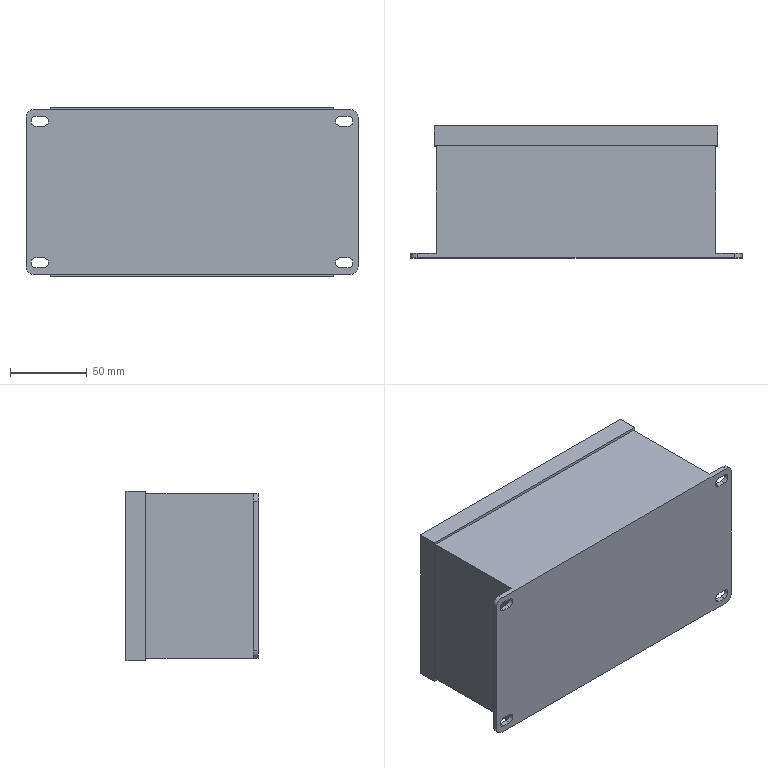Part | SolidWorks | features ICE 2, Extrusion 1 | 1 solid | 35 faces | box 216 x 86 x 110.411 mm | volume 1696161 mm3 | plane 23 | cylinder 12 | commonest cylinder face diameters 6.4 x8 10 x4
STEP:
#1=CARTESIAN_POINT('',(96.5,3.,42.8));
#2=VERTEX_POINT('',#1);
#3=CARTESIAN_POINT('',(96.5,3.,49.2));
#4=VERTEX_POINT('',#3);
#5=CARTESIAN_POINT('',(96.5,3.,46.));
#6=DIRECTION('',(0.,1.,0.));
#7=DIRECTION('',(0.,0.,1.));
#8=AXIS2_PLACEMENT_3D('',#5,#6,#7);
#9=CIRCLE('',#8,3.2);
#10=EDGE_CURVE('',#2,#4,#9,.T.);
#11=ORIENTED_EDGE('',*,*,#10,.F.);
#12=CARTESIAN_POINT('',(101.5,3.,42.8));
#13=VERTEX_POINT('',#12);
#14=CARTESIAN_POINT('',(96.5,3.,42.8));
#15=DIRECTION('',(-1.,0.,0.));
#16=VECTOR('',#15,1000.);
#17=LINE('',#14,#16);
#18=EDGE_CURVE('',#13,#2,#17,.T.);
#19=ORIENTED_EDGE('',*,*,#18,.F.);
#20=CARTESIAN_POINT('',(101.5,3.,49.2));
#21=VERTEX_POINT('',#20);
#22=CARTESIAN_POINT('',(101.5,3.,46.));
#23=DIRECTION('',(0.,1.,0.));
#24=DIRECTION('',(0.,0.,1.));
#25=AXIS2_PLACEMENT_3D('',#22,#23,#24);
#26=CIRCLE('',#25,3.2);
#27=EDGE_CURVE('',#21,#13,#26,.T.);
#28=ORIENTED_EDGE('',*,*,#27,.F.);
#29=CARTESIAN_POINT('',(96.5,3.,49.2));
#30=DIRECTION('',(1.,0.,0.));
#31=VECTOR('',#30,1000.);
#32=LINE('',#29,#31);
#33=EDGE_CURVE('',#4,#21,#32,.T.);
#34=ORIENTED_EDGE('',*,*,#33,.F.);
#35=EDGE_LOOP('',(#11,#19,#28,#34));
#36=FACE_BOUND('',#35,.T.);
#37=CARTESIAN_POINT('',(96.5,3.,-49.2));
#38=VERTEX_POINT('',#37);
#39=CARTESIAN_POINT('',(96.5,3.,-42.8));
#40=VERTEX_POINT('',#39);
#41=CARTESIAN_POINT('',(96.5,3.,-46.));
#42=DIRECTION('',(0.,1.,0.));
#43=DIRECTION('',(0.,0.,1.));
#44=AXIS2_PLACEMENT_3D('',#41,#42,#43);
#45=CIRCLE('',#44,3.2);
#46=EDGE_CURVE('',#38,#40,#45,.T.);
#47=ORIENTED_EDGE('',*,*,#46,.F.);
#48=CARTESIAN_POINT('',(101.5,3.,-49.2));
#49=VERTEX_POINT('',#48);
#50=CARTESIAN_POINT('',(96.5,3.,-49.2));
#51=DIRECTION('',(-1.,0.,0.));
#52=VECTOR('',#51,1000.);
#53=LINE('',#50,#52);
#54=EDGE_CURVE('',#49,#38,#53,.T.);
#55=ORIENTED_EDGE('',*,*,#54,.F.);
#56=CARTESIAN_POINT('',(101.5,3.,-42.8));
#57=VERTEX_POINT('',#56);
#58=CARTESIAN_POINT('',(101.5,3.,-46.));
#59=DIRECTION('',(0.,1.,0.));
#60=DIRECTION('',(0.,0.,1.));
#61=AXIS2_PLACEMENT_3D('',#58,#59,#60);
#62=CIRCLE('',#61,3.2);
#63=EDGE_CURVE('',#57,#49,#62,.T.);
#64=ORIENTED_EDGE('',*,*,#63,.F.);
#65=CARTESIAN_POINT('',(96.5,3.,-42.8));
#66=DIRECTION('',(1.,0.,0.));
#67=VECTOR('',#66,1000.);
#68=LINE('',#65,#67);
#69=EDGE_CURVE('',#40,#57,#68,.T.);
#70=ORIENTED_EDGE('',*,*,#69,.F.);
#71=EDGE_LOOP('',(#47,#55,#64,#70));
#72=FACE_BOUND('',#71,.T.);
#73=CARTESIAN_POINT('',(91.,3.,53.5));
#74=VERTEX_POINT('',#73);
#75=CARTESIAN_POINT('',(91.,3.,-53.5));
#76=VERTEX_POINT('',#75);
#77=CARTESIAN_POINT('',(91.,3.,53.5));
#78=DIRECTION('',(0.,0.,-1.));
#79=VECTOR('',#78,1000.);
#80=LINE('',#77,#79);
#81=EDGE_CURVE('',#74,#76,#80,.T.);
#82=ORIENTED_EDGE('',*,*,#81,.F.);
#83=CARTESIAN_POINT('',(103.,3.,53.5));
#84=VERTEX_POINT('',#83);
#85=CARTESIAN_POINT('',(-103.,3.,53.5));
#86=DIRECTION('',(1.,0.,0.));
#87=VECTOR('',#86,1000.);
#88=LINE('',#85,#87);
#89=EDGE_CURVE('',#74,#84,#88,.T.);
#90=ORIENTED_EDGE('',*,*,#89,.T.);
#91=CARTESIAN_POINT('',(108.,3.,48.5));
#92=VERTEX_POINT('',#91);
#93=CARTESIAN_POINT('',(103.,3.,48.5));
#94=DIRECTION('',(0.,1.,0.));
#95=DIRECTION('',(0.,0.,1.));
#96=AXIS2_PLACEMENT_3D('',#93,#94,#95);
#97=CIRCLE('',#96,5.);
#98=EDGE_CURVE('',#84,#92,#97,.T.);
#99=ORIENTED_EDGE('',*,*,#98,.T.);
#100=CARTESIAN_POINT('',(108.,3.,-48.5));
#101=VERTEX_POINT('',#100);
#102=CARTESIAN_POINT('',(108.,3.,48.5));
#103=DIRECTION('',(0.,0.,-1.));
#104=VECTOR('',#103,1000.);
#105=LINE('',#102,#104);
#106=EDGE_CURVE('',#92,#101,#105,.T.);
#107=ORIENTED_EDGE('',*,*,#106,.T.);
#108=CARTESIAN_POINT('',(103.,3.,-53.5));
#109=VERTEX_POINT('',#108);
#110=CARTESIAN_POINT('',(103.,3.,-48.5));
#111=DIRECTION('',(0.,1.,0.));
#112=DIRECTION('',(0.,0.,-1.));
#113=AXIS2_PLACEMENT_3D('',#110,#111,#112);
#114=CIRCLE('',#113,5.);
#115=EDGE_CURVE('',#101,#109,#114,.T.);
#116=ORIENTED_EDGE('',*,*,#115,.T.);
#117=CARTESIAN_POINT('',(-103.,3.,-53.5));
#118=DIRECTION('',(-1.,0.,0.));
#119=VECTOR('',#118,1000.);
#120=LINE('',#117,#119);
#121=EDGE_CURVE('',#109,#76,#120,.T.);
#122=ORIENTED_EDGE('',*,*,#121,.T.);
#123=EDGE_LOOP('',(#82,#90,#99,#107,#116,#122));
#124=FACE_OUTER_BOUND('',#123,.T.);
#125=CARTESIAN_POINT('',(-103.,3.,48.5));
#126=DIRECTION('',(0.,-1.,0.));
#127=DIRECTION('',(0.,0.,-1.));
#128=AXIS2_PLACEMENT_3D('',#125,#126,#127);
#129=PLANE('',#128);
#130=ADVANCED_FACE('',(#36,#72,#124),#129,.F.);
#131=CARTESIAN_POINT('',(-101.5,3.,-49.2));
#132=VERTEX_POINT('',#131);
#133=CARTESIAN_POINT('',(-101.5,3.,-42.8));
#134=VERTEX_POINT('',#133);
#135=CARTESIAN_POINT('',(-101.5,3.,-46.));
#136=DIRECTION('',(0.,1.,0.));
#137=DIRECTION('',(0.,0.,1.));
#138=AXIS2_PLACEMENT_3D('',#135,#136,#137);
#139=CIRCLE('',#138,3.2);
#140=EDGE_CURVE('',#132,#134,#139,.T.);
#141=ORIENTED_EDGE('',*,*,#140,.F.);
#142=CARTESIAN_POINT('',(-96.5,3.,-49.2));
#143=VERTEX_POINT('',#142);
#144=CARTESIAN_POINT('',(-101.5,3.,-49.2));
#145=DIRECTION('',(-1.,0.,0.));
#146=VECTOR('',#145,1000.);
#147=LINE('',#144,#146);
#148=EDGE_CURVE('',#143,#132,#147,.T.);
#149=ORIENTED_EDGE('',*,*,#148,.F.);
#150=CARTESIAN_POINT('',(-96.5,3.,-42.8));
#151=VERTEX_POINT('',#150);
#152=CARTESIAN_POINT('',(-96.5,3.,-46.));
#153=DIRECTION('',(0.,1.,0.));
#154=DIRECTION('',(0.,0.,1.));
#155=AXIS2_PLACEMENT_3D('',#152,#153,#154);
#156=CIRCLE('',#155,3.2);
#157=EDGE_CURVE('',#151,#143,#156,.T.);
#158=ORIENTED_EDGE('',*,*,#157,.F.);
#159=CARTESIAN_POINT('',(-101.5,3.,-42.8));
#160=DIRECTION('',(1.,0.,0.));
#161=VECTOR('',#160,1000.);
#162=LINE('',#159,#161);
#163=EDGE_CURVE('',#134,#151,#162,.T.);
#164=ORIENTED_EDGE('',*,*,#163,.F.);
#165=EDGE_LOOP('',(#141,#149,#158,#164));
#166=FACE_BOUND('',#165,.T.);
#167=CARTESIAN_POINT('',(-101.5,3.,42.8));
#168=VERTEX_POINT('',#167);
#169=CARTESIAN_POINT('',(-101.5,3.,49.2));
#170=VERTEX_POINT('',#169);
#171=CARTESIAN_POINT('',(-101.5,3.,46.));
#172=DIRECTION('',(0.,1.,0.));
#173=DIRECTION('',(0.,0.,1.));
#174=AXIS2_PLACEMENT_3D('',#171,#172,#173);
#175=CIRCLE('',#174,3.2);
#176=EDGE_CURVE('',#168,#170,#175,.T.);
#177=ORIENTED_EDGE('',*,*,#176,.F.);
#178=CARTESIAN_POINT('',(-96.5,3.,42.8));
#179=VERTEX_POINT('',#178);
#180=CARTESIAN_POINT('',(-101.5,3.,42.8));
#181=DIRECTION('',(-1.,0.,0.));
#182=VECTOR('',#181,1000.);
#183=LINE('',#180,#182);
#184=EDGE_CURVE('',#179,#168,#183,.T.);
#185=ORIENTED_EDGE('',*,*,#184,.F.);
#186=CARTESIAN_POINT('',(-96.5,3.,49.2));
#187=VERTEX_POINT('',#186);
#188=CARTESIAN_POINT('',(-96.5,3.,46.));
#189=DIRECTION('',(0.,1.,0.));
#190=DIRECTION('',(0.,0.,1.));
#191=AXIS2_PLACEMENT_3D('',#188,#189,#190);
#192=CIRCLE('',#191,3.2);
#193=EDGE_CURVE('',#187,#179,#192,.T.);
#194=ORIENTED_EDGE('',*,*,#193,.F.);
#195=CARTESIAN_POINT('',(-101.5,3.,49.2));
#196=DIRECTION('',(1.,0.,0.));
#197=VECTOR('',#196,1000.);
#198=LINE('',#195,#197);
#199=EDGE_CURVE('',#170,#187,#198,.T.);
#200=ORIENTED_EDGE('',*,*,#199,.F.);
#201=EDGE_LOOP('',(#177,#185,#194,#200));
#202=FACE_BOUND('',#201,.T.);
#203=CARTESIAN_POINT('',(-91.,3.,-53.5));
#204=VERTEX_POINT('',#203);
#205=CARTESIAN_POINT('',(-91.,3.,53.5));
#206=VERTEX_POINT('',#205);
#207=CARTESIAN_POINT('',(-91.,3.,53.5));
#208=DIRECTION('',(0.,0.,1.));
#209=VECTOR('',#208,1000.);
#210=LINE('',#207,#209);
#211=EDGE_CURVE('',#204,#206,#210,.T.);
#212=ORIENTED_EDGE('',*,*,#211,.F.);
#213=CARTESIAN_POINT('',(-103.,3.,-53.5));
#214=VERTEX_POINT('',#213);
#215=CARTESIAN_POINT('',(-103.,3.,-53.5));
#216=DIRECTION('',(-1.,0.,0.));
#217=VECTOR('',#216,1000.);
#218=LINE('',#215,#217);
#219=EDGE_CURVE('',#204,#214,#218,.T.);
#220=ORIENTED_EDGE('',*,*,#219,.T.);
#221=CARTESIAN_POINT('',(-108.,3.,-48.5));
#222=VERTEX_POINT('',#221);
#223=CARTESIAN_POINT('',(-103.,3.,-48.5));
#224=DIRECTION('',(0.,1.,0.));
#225=DIRECTION('',(0.,0.,-1.));
#226=AXIS2_PLACEMENT_3D('',#223,#224,#225);
#227=CIRCLE('',#226,5.);
#228=EDGE_CURVE('',#214,#222,#227,.T.);
#229=ORIENTED_EDGE('',*,*,#228,.T.);
#230=CARTESIAN_POINT('',(-108.,3.,48.5));
#231=VERTEX_POINT('',#230);
#232=CARTESIAN_POINT('',(-108.,3.,48.5));
#233=DIRECTION('',(0.,0.,1.));
#234=VECTOR('',#233,1000.);
#235=LINE('',#232,#234);
#236=EDGE_CURVE('',#222,#231,#235,.T.);
#237=ORIENTED_EDGE('',*,*,#236,.T.);
#238=CARTESIAN_POINT('',(-103.,3.,53.5));
#239=VERTEX_POINT('',#238);
#240=CARTESIAN_POINT('',(-103.,3.,48.5));
#241=DIRECTION('',(0.,1.,0.));
#242=DIRECTION('',(0.,0.,-1.));
#243=AXIS2_PLACEMENT_3D('',#240,#241,#242);
#244=CIRCLE('',#243,5.);
#245=EDGE_CURVE('',#231,#239,#244,.T.);
#246=ORIENTED_EDGE('',*,*,#245,.T.);
#247=CARTESIAN_POINT('',(-103.,3.,53.5));
#248=DIRECTION('',(1.,0.,0.));
#249=VECTOR('',#248,1000.);
#250=LINE('',#247,#249);
#251=EDGE_CURVE('',#239,#206,#250,.T.);
#252=ORIENTED_EDGE('',*,*,#251,.T.);
#253=EDGE_LOOP('',(#212,#220,#229,#237,#246,#252));
#254=FACE_OUTER_BOUND('',#253,.T.);
#255=CARTESIAN_POINT('',(-103.,3.,48.5));
#256=DIRECTION('',(0.,-1.,0.));
#257=DIRECTION('',(0.,0.,-1.));
#258=AXIS2_PLACEMENT_3D('',#255,#256,#257);
#259=PLANE('',#258);
#260=ADVANCED_FACE('',(#166,#202,#254),#259,.F.);
#261=CARTESIAN_POINT('',(-108.,0.,48.5));
#262=VERTEX_POINT('',#261);
#263=CARTESIAN_POINT('',(-103.,0.,53.5));
#264=VERTEX_POINT('',#263);
#265=CARTESIAN_POINT('',(-103.,0.,48.5));
#266=DIRECTION('',(0.,1.,0.));
#267=DIRECTION('',(0.,0.,-1.));
#268=AXIS2_PLACEMENT_3D('',#265,#266,#267);
#269=CIRCLE('',#268,5.);
#270=EDGE_CURVE('',#262,#264,#269,.T.);
#271=ORIENTED_EDGE('',*,*,#270,.F.);
#272=CARTESIAN_POINT('',(-108.,0.,-48.5));
#273=VERTEX_POINT('',#272);
#274=CARTESIAN_POINT('',(-108.,0.,48.5));
#275=DIRECTION('',(0.,0.,1.));
#276=VECTOR('',#275,1000.);
#277=LINE('',#274,#276);
#278=EDGE_CURVE('',#273,#262,#277,.T.);
#279=ORIENTED_EDGE('',*,*,#278,.F.);
#280=CARTESIAN_POINT('',(-103.,0.,-53.5));
#281=VERTEX_POINT('',#280);
#282=CARTESIAN_POINT('',(-103.,0.,-48.5));
#283=DIRECTION('',(0.,1.,0.));
#284=DIRECTION('',(0.,0.,-1.));
#285=AXIS2_PLACEMENT_3D('',#282,#283,#284);
#286=CIRCLE('',#285,5.);
#287=EDGE_CURVE('',#281,#273,#286,.T.);
#288=ORIENTED_EDGE('',*,*,#287,.F.);
#289=CARTESIAN_POINT('',(103.,0.,-53.5));
#290=VERTEX_POINT('',#289);
#291=CARTESIAN_POINT('',(-103.,0.,-53.5));
#292=DIRECTION('',(-1.,0.,0.));
#293=VECTOR('',#292,1000.);
#294=LINE('',#291,#293);
#295=EDGE_CURVE('',#290,#281,#294,.T.);
#296=ORIENTED_EDGE('',*,*,#295,.F.);
#297=CARTESIAN_POINT('',(108.,0.,-48.5));
#298=VERTEX_POINT('',#297);
#299=CARTESIAN_POINT('',(103.,0.,-48.5));
#300=DIRECTION('',(0.,1.,0.));
#301=DIRECTION('',(0.,0.,-1.));
#302=AXIS2_PLACEMENT_3D('',#299,#300,#301);
#303=CIRCLE('',#302,5.);
#304=EDGE_CURVE('',#298,#290,#303,.T.);
#305=ORIENTED_EDGE('',*,*,#304,.F.);
#306=CARTESIAN_POINT('',(108.,0.,48.5));
#307=VERTEX_POINT('',#306);
#308=CARTESIAN_POINT('',(108.,0.,48.5));
#309=DIRECTION('',(0.,0.,-1.));
#310=VECTOR('',#309,1000.);
#311=LINE('',#308,#310);
#312=EDGE_CURVE('',#307,#298,#311,.T.);
#313=ORIENTED_EDGE('',*,*,#312,.F.);
#314=CARTESIAN_POINT('',(103.,0.,53.5));
#315=VERTEX_POINT('',#314);
#316=CARTESIAN_POINT('',(103.,0.,48.5));
#317=DIRECTION('',(0.,1.,0.));
#318=DIRECTION('',(0.,0.,1.));
#319=AXIS2_PLACEMENT_3D('',#316,#317,#318);
#320=CIRCLE('',#319,5.);
#321=EDGE_CURVE('',#315,#307,#320,.T.);
#322=ORIENTED_EDGE('',*,*,#321,.F.);
#323=CARTESIAN_POINT('',(-103.,0.,53.5));
#324=DIRECTION('',(1.,0.,0.));
#325=VECTOR('',#324,1000.);
#326=LINE('',#323,#325);
#327=EDGE_CURVE('',#264,#315,#326,.T.);
#328=ORIENTED_EDGE('',*,*,#327,.F.);
#329=EDGE_LOOP('',(#271,#279,#288,#296,#305,#313,#322,#328));
#330=FACE_OUTER_BOUND('',#329,.T.);
#331=CARTESIAN_POINT('',(-96.5,0.,-49.2));
#332=VERTEX_POINT('',#331);
#333=CARTESIAN_POINT('',(-101.5,0.,-49.2));
#334=VERTEX_POINT('',#333);
#335=CARTESIAN_POINT('',(-101.5,0.,-49.2));
#336=DIRECTION('',(-1.,0.,0.));
#337=VECTOR('',#336,1000.);
#338=LINE('',#335,#337);
#339=EDGE_CURVE('',#332,#334,#338,.T.);
#340=ORIENTED_EDGE('',*,*,#339,.T.);
#341=CARTESIAN_POINT('',(-101.5,0.,-42.8));
#342=VERTEX_POINT('',#341);
#343=CARTESIAN_POINT('',(-101.5,0.,-46.));
#344=DIRECTION('',(0.,1.,0.));
#345=DIRECTION('',(0.,0.,1.));
#346=AXIS2_PLACEMENT_3D('',#343,#344,#345);
#347=CIRCLE('',#346,3.2);
#348=EDGE_CURVE('',#334,#342,#347,.T.);
#349=ORIENTED_EDGE('',*,*,#348,.T.);
#350=CARTESIAN_POINT('',(-96.5,0.,-42.8));
#351=VERTEX_POINT('',#350);
#352=CARTESIAN_POINT('',(-101.5,0.,-42.8));
#353=DIRECTION('',(1.,0.,0.));
#354=VECTOR('',#353,1000.);
#355=LINE('',#352,#354);
#356=EDGE_CURVE('',#342,#351,#355,.T.);
#357=ORIENTED_EDGE('',*,*,#356,.T.);
#358=CARTESIAN_POINT('',(-96.5,0.,-46.));
#359=DIRECTION('',(0.,1.,0.));
#360=DIRECTION('',(0.,0.,1.));
#361=AXIS2_PLACEMENT_3D('',#358,#359,#360);
#362=CIRCLE('',#361,3.2);
#363=EDGE_CURVE('',#351,#332,#362,.T.);
#364=ORIENTED_EDGE('',*,*,#363,.T.);
#365=EDGE_LOOP('',(#340,#349,#357,#364));
#366=FACE_BOUND('',#365,.T.);
#367=CARTESIAN_POINT('',(101.5,0.,-49.2));
#368=VERTEX_POINT('',#367);
#369=CARTESIAN_POINT('',(96.5,0.,-49.2));
#370=VERTEX_POINT('',#369);
#371=CARTESIAN_POINT('',(96.5,0.,-49.2));
#372=DIRECTION('',(-1.,0.,0.));
#373=VECTOR('',#372,1000.);
#374=LINE('',#371,#373);
#375=EDGE_CURVE('',#368,#370,#374,.T.);
#376=ORIENTED_EDGE('',*,*,#375,.T.);
#377=CARTESIAN_POINT('',(96.5,0.,-42.8));
#378=VERTEX_POINT('',#377);
#379=CARTESIAN_POINT('',(96.5,0.,-46.));
#380=DIRECTION('',(0.,1.,0.));
#381=DIRECTION('',(0.,0.,1.));
#382=AXIS2_PLACEMENT_3D('',#379,#380,#381);
#383=CIRCLE('',#382,3.2);
#384=EDGE_CURVE('',#370,#378,#383,.T.);
#385=ORIENTED_EDGE('',*,*,#384,.T.);
#386=CARTESIAN_POINT('',(101.5,0.,-42.8));
#387=VERTEX_POINT('',#386);
#388=CARTESIAN_POINT('',(96.5,0.,-42.8));
#389=DIRECTION('',(1.,0.,0.));
#390=VECTOR('',#389,1000.);
#391=LINE('',#388,#390);
#392=EDGE_CURVE('',#378,#387,#391,.T.);
#393=ORIENTED_EDGE('',*,*,#392,.T.);
#394=CARTESIAN_POINT('',(101.5,0.,-46.));
#395=DIRECTION('',(0.,1.,0.));
#396=DIRECTION('',(0.,0.,1.));
#397=AXIS2_PLACEMENT_3D('',#394,#395,#396);
#398=CIRCLE('',#397,3.2);
#399=EDGE_CURVE('',#387,#368,#398,.T.);
#400=ORIENTED_EDGE('',*,*,#399,.T.);
#401=EDGE_LOOP('',(#376,#385,#393,#400));
#402=FACE_BOUND('',#401,.T.);
#403=CARTESIAN_POINT('',(-96.5,0.,42.8));
#404=VERTEX_POINT('',#403);
#405=CARTESIAN_POINT('',(-101.5,0.,42.8));
#406=VERTEX_POINT('',#405);
#407=CARTESIAN_POINT('',(-101.5,0.,42.8));
#408=DIRECTION('',(-1.,0.,0.));
#409=VECTOR('',#408,1000.);
#410=LINE('',#407,#409);
#411=EDGE_CURVE('',#404,#406,#410,.T.);
#412=ORIENTED_EDGE('',*,*,#411,.T.);
#413=CARTESIAN_POINT('',(-101.5,0.,49.2));
#414=VERTEX_POINT('',#413);
#415=CARTESIAN_POINT('',(-101.5,0.,46.));
#416=DIRECTION('',(0.,1.,0.));
#417=DIRECTION('',(0.,0.,1.));
#418=AXIS2_PLACEMENT_3D('',#415,#416,#417);
#419=CIRCLE('',#418,3.2);
#420=EDGE_CURVE('',#406,#414,#419,.T.);
#421=ORIENTED_EDGE('',*,*,#420,.T.);
#422=CARTESIAN_POINT('',(-96.5,0.,49.2));
#423=VERTEX_POINT('',#422);
#424=CARTESIAN_POINT('',(-101.5,0.,49.2));
#425=DIRECTION('',(1.,0.,0.));
#426=VECTOR('',#425,1000.);
#427=LINE('',#424,#426);
#428=EDGE_CURVE('',#414,#423,#427,.T.);
#429=ORIENTED_EDGE('',*,*,#428,.T.);
#430=CARTESIAN_POINT('',(-96.5,0.,46.));
#431=DIRECTION('',(0.,1.,0.));
#432=DIRECTION('',(0.,0.,1.));
#433=AXIS2_PLACEMENT_3D('',#430,#431,#432);
#434=CIRCLE('',#433,3.2);
#435=EDGE_CURVE('',#423,#404,#434,.T.);
#436=ORIENTED_EDGE('',*,*,#435,.T.);
#437=EDGE_LOOP('',(#412,#421,#429,#436));
#438=FACE_BOUND('',#437,.T.);
#439=CARTESIAN_POINT('',(101.5,0.,42.8));
#440=VERTEX_POINT('',#439);
#441=CARTESIAN_POINT('',(96.5,0.,42.8));
#442=VERTEX_POINT('',#441);
#443=CARTESIAN_POINT('',(96.5,0.,42.8));
#444=DIRECTION('',(-1.,0.,0.));
#445=VECTOR('',#444,1000.);
#446=LINE('',#443,#445);
#447=EDGE_CURVE('',#440,#442,#446,.T.);
#448=ORIENTED_EDGE('',*,*,#447,.T.);
#449=CARTESIAN_POINT('',(96.5,0.,49.2));
#450=VERTEX_POINT('',#449);
#451=CARTESIAN_POINT('',(96.5,0.,46.));
#452=DIRECTION('',(0.,1.,0.));
#453=DIRECTION('',(0.,0.,1.));
#454=AXIS2_PLACEMENT_3D('',#451,#452,#453);
#455=CIRCLE('',#454,3.2);
#456=EDGE_CURVE('',#442,#450,#455,.T.);
#457=ORIENTED_EDGE('',*,*,#456,.T.);
#458=CARTESIAN_POINT('',(101.5,0.,49.2));
#459=VERTEX_POINT('',#458);
#460=CARTESIAN_POINT('',(96.5,0.,49.2));
#461=DIRECTION('',(1.,0.,0.));
#462=VECTOR('',#461,1000.);
#463=LINE('',#460,#462);
#464=EDGE_CURVE('',#450,#459,#463,.T.);
#465=ORIENTED_EDGE('',*,*,#464,.T.);
#466=CARTESIAN_POINT('',(101.5,0.,46.));
#467=DIRECTION('',(0.,1.,0.));
#468=DIRECTION('',(0.,0.,1.));
#469=AXIS2_PLACEMENT_3D('',#466,#467,#468);
#470=CIRCLE('',#469,3.2);
#471=EDGE_CURVE('',#459,#440,#470,.T.);
#472=ORIENTED_EDGE('',*,*,#471,.T.);
#473=EDGE_LOOP('',(#448,#457,#465,#472));
#474=FACE_BOUND('',#473,.T.);
#475=CARTESIAN_POINT('',(-103.,0.,48.5));
#476=DIRECTION('',(0.,-1.,0.));
#477=DIRECTION('',(0.,0.,-1.));
#478=AXIS2_PLACEMENT_3D('',#475,#476,#477);
#479=PLANE('',#478);
#480=ADVANCED_FACE('',(#330,#366,#402,#438,#474),#479,.T.);
#481=ORIENTED_EDGE('',*,*,#270,.T.);
#482=CARTESIAN_POINT('',(-103.,3.,53.5));
#483=DIRECTION('',(0.,-1.,0.));
#484=VECTOR('',#483,1000.);
#485=LINE('',#482,#484);
#486=EDGE_CURVE('',#239,#264,#485,.T.);
#487=ORIENTED_EDGE('',*,*,#486,.F.);
#488=ORIENTED_EDGE('',*,*,#245,.F.);
#489=CARTESIAN_POINT('',(-108.,3.,48.5));
#490=DIRECTION('',(0.,-1.,0.));
#491=VECTOR('',#490,1000.);
#492=LINE('',#489,#491);
#493=EDGE_CURVE('',#231,#262,#492,.T.);
#494=ORIENTED_EDGE('',*,*,#493,.T.);
#495=EDGE_LOOP('',(#481,#487,#488,#494));
#496=FACE_OUTER_BOUND('',#495,.T.);
#497=CARTESIAN_POINT('',(-103.,3.,48.5));
#498=DIRECTION('',(0.,-1.,0.));
#499=DIRECTION('',(0.,0.,-1.));
#500=AXIS2_PLACEMENT_3D('',#497,#498,#499);
#501=CYLINDRICAL_SURFACE('',#500,5.);
#502=ADVANCED_FACE('',(#496),#501,.T.);
#503=ORIENTED_EDGE('',*,*,#327,.T.);
#504=CARTESIAN_POINT('',(103.,3.,53.5));
#505=DIRECTION('',(0.,-1.,0.));
#506=VECTOR('',#505,1000.);
#507=LINE('',#504,#506);
#508=EDGE_CURVE('',#84,#315,#507,.T.);
#509=ORIENTED_EDGE('',*,*,#508,.F.);
#510=ORIENTED_EDGE('',*,*,#89,.F.);
#511=CARTESIAN_POINT('',(91.,73.,53.5));
#512=VERTEX_POINT('',#511);
#513=CARTESIAN_POINT('',(91.,73.,53.5));
#514=DIRECTION('',(0.,-1.,0.));
#515=VECTOR('',#514,1000.);
#516=LINE('',#513,#515);
#517=EDGE_CURVE('',#512,#74,#516,.T.);
#518=ORIENTED_EDGE('',*,*,#517,.F.);
#519=CARTESIAN_POINT('',(-91.,73.,53.5));
#520=VERTEX_POINT('',#519);
#521=CARTESIAN_POINT('',(-91.,73.,53.5));
#522=DIRECTION('',(1.,0.,0.));
#523=VECTOR('',#522,1000.);
#524=LINE('',#521,#523);
#525=EDGE_CURVE('',#520,#512,#524,.T.);
#526=ORIENTED_EDGE('',*,*,#525,.F.);
#527=CARTESIAN_POINT('',(-91.,73.,53.5));
#528=DIRECTION('',(0.,-1.,0.));
#529=VECTOR('',#528,1000.);
#530=LINE('',#527,#529);
#531=EDGE_CURVE('',#520,#206,#530,.T.);
#532=ORIENTED_EDGE('',*,*,#531,.T.);
#533=ORIENTED_EDGE('',*,*,#251,.F.);
#534=ORIENTED_EDGE('',*,*,#486,.T.);
#535=EDGE_LOOP('',(#503,#509,#510,#518,#526,#532,#533,#534));
#536=FACE_OUTER_BOUND('',#535,.T.);
#537=CARTESIAN_POINT('',(-103.,3.,53.5));
#538=DIRECTION('',(0.,0.,-1.));
#539=DIRECTION('',(-1.,0.,0.));
#540=AXIS2_PLACEMENT_3D('',#537,#538,#539);
#541=PLANE('',#540);
#542=ADVANCED_FACE('',(#536),#541,.F.);
#543=ORIENTED_EDGE('',*,*,#321,.T.);
#544=CARTESIAN_POINT('',(108.,3.,48.5));
#545=DIRECTION('',(0.,-1.,0.));
#546=VECTOR('',#545,1000.);
#547=LINE('',#544,#546);
#548=EDGE_CURVE('',#92,#307,#547,.T.);
#549=ORIENTED_EDGE('',*,*,#548,.F.);
#550=ORIENTED_EDGE('',*,*,#98,.F.);
#551=ORIENTED_EDGE('',*,*,#508,.T.);
#552=EDGE_LOOP('',(#543,#549,#550,#551));
#553=FACE_OUTER_BOUND('',#552,.T.);
#554=CARTESIAN_POINT('',(103.,3.,48.5));
#555=DIRECTION('',(0.,-1.,0.));
#556=DIRECTION('',(0.,0.,-1.));
#557=AXIS2_PLACEMENT_3D('',#554,#555,#556);
#558=CYLINDRICAL_SURFACE('',#557,5.);
#559=ADVANCED_FACE('',(#553),#558,.T.);
#560=ORIENTED_EDGE('',*,*,#312,.T.);
#561=CARTESIAN_POINT('',(108.,3.,-48.5));
#562=DIRECTION('',(0.,-1.,0.));
#563=VECTOR('',#562,1000.);
#564=LINE('',#561,#563);
#565=EDGE_CURVE('',#101,#298,#564,.T.);
#566=ORIENTED_EDGE('',*,*,#565,.F.);
#567=ORIENTED_EDGE('',*,*,#106,.F.);
#568=ORIENTED_EDGE('',*,*,#548,.T.);
#569=EDGE_LOOP('',(#560,#566,#567,#568));
#570=FACE_OUTER_BOUND('',#569,.T.);
#571=CARTESIAN_POINT('',(108.,3.,48.5));
#572=DIRECTION('',(-1.,0.,0.));
#573=DIRECTION('',(0.,0.,1.));
#574=AXIS2_PLACEMENT_3D('',#571,#572,#573);
#575=PLANE('',#574);
#576=ADVANCED_FACE('',(#570),#575,.F.);
#577=ORIENTED_EDGE('',*,*,#304,.T.);
#578=CARTESIAN_POINT('',(103.,3.,-53.5));
#579=DIRECTION('',(0.,-1.,0.));
#580=VECTOR('',#579,1000.);
#581=LINE('',#578,#580);
#582=EDGE_CURVE('',#109,#290,#581,.T.);
#583=ORIENTED_EDGE('',*,*,#582,.F.);
#584=ORIENTED_EDGE('',*,*,#115,.F.);
#585=ORIENTED_EDGE('',*,*,#565,.T.);
#586=EDGE_LOOP('',(#577,#583,#584,#585));
#587=FACE_OUTER_BOUND('',#586,.T.);
#588=CARTESIAN_POINT('',(103.,3.,-48.5));
#589=DIRECTION('',(0.,-1.,0.));
#590=DIRECTION('',(0.,0.,-1.));
#591=AXIS2_PLACEMENT_3D('',#588,#589,#590);
#592=CYLINDRICAL_SURFACE('',#591,5.);
#593=ADVANCED_FACE('',(#587),#592,.T.);
#594=ORIENTED_EDGE('',*,*,#295,.T.);
#595=CARTESIAN_POINT('',(-103.,3.,-53.5));
#596=DIRECTION('',(0.,-1.,0.));
#597=VECTOR('',#596,1000.);
#598=LINE('',#595,#597);
#599=EDGE_CURVE('',#214,#281,#598,.T.);
#600=ORIENTED_EDGE('',*,*,#599,.F.);
#601=ORIENTED_EDGE('',*,*,#219,.F.);
#602=CARTESIAN_POINT('',(-91.,73.,-53.5));
#603=VERTEX_POINT('',#602);
#604=CARTESIAN_POINT('',(-91.,73.,-53.5));
#605=DIRECTION('',(0.,-1.,0.));
#606=VECTOR('',#605,1000.);
#607=LINE('',#604,#606);
#608=EDGE_CURVE('',#603,#204,#607,.T.);
#609=ORIENTED_EDGE('',*,*,#608,.F.);
#610=CARTESIAN_POINT('',(91.,73.,-53.5));
#611=VERTEX_POINT('',#610);
#612=CARTESIAN_POINT('',(-91.,73.,-53.5));
#613=DIRECTION('',(-1.,0.,0.));
#614=VECTOR('',#613,1000.);
#615=LINE('',#612,#614);
#616=EDGE_CURVE('',#611,#603,#615,.T.);
#617=ORIENTED_EDGE('',*,*,#616,.F.);
#618=CARTESIAN_POINT('',(91.,73.,-53.5));
#619=DIRECTION('',(0.,-1.,0.));
#620=VECTOR('',#619,1000.);
#621=LINE('',#618,#620);
#622=EDGE_CURVE('',#611,#76,#621,.T.);
#623=ORIENTED_EDGE('',*,*,#622,.T.);
#624=ORIENTED_EDGE('',*,*,#121,.F.);
#625=ORIENTED_EDGE('',*,*,#582,.T.);
#626=EDGE_LOOP('',(#594,#600,#601,#609,#617,#623,#624,#625));
#627=FACE_OUTER_BOUND('',#626,.T.);
#628=CARTESIAN_POINT('',(-103.,3.,-53.5));
#629=DIRECTION('',(0.,0.,1.));
#630=DIRECTION('',(1.,0.,0.));
#631=AXIS2_PLACEMENT_3D('',#628,#629,#630);
#632=PLANE('',#631);
#633=ADVANCED_FACE('',(#627),#632,.F.);
#634=ORIENTED_EDGE('',*,*,#287,.T.);
#635=CARTESIAN_POINT('',(-108.,3.,-48.5));
#636=DIRECTION('',(0.,-1.,0.));
#637=VECTOR('',#636,1000.);
#638=LINE('',#635,#637);
#639=EDGE_CURVE('',#222,#273,#638,.T.);
#640=ORIENTED_EDGE('',*,*,#639,.F.);
#641=ORIENTED_EDGE('',*,*,#228,.F.);
#642=ORIENTED_EDGE('',*,*,#599,.T.);
#643=EDGE_LOOP('',(#634,#640,#641,#642));
#644=FACE_OUTER_BOUND('',#643,.T.);
#645=CARTESIAN_POINT('',(-103.,3.,-48.5));
#646=DIRECTION('',(0.,-1.,0.));
#647=DIRECTION('',(0.,0.,-1.));
#648=AXIS2_PLACEMENT_3D('',#645,#646,#647);
#649=CYLINDRICAL_SURFACE('',#648,5.);
#650=ADVANCED_FACE('',(#644),#649,.T.);
#651=ORIENTED_EDGE('',*,*,#278,.T.);
#652=ORIENTED_EDGE('',*,*,#493,.F.);
#653=ORIENTED_EDGE('',*,*,#236,.F.);
#654=ORIENTED_EDGE('',*,*,#639,.T.);
#655=EDGE_LOOP('',(#651,#652,#653,#654));
#656=FACE_OUTER_BOUND('',#655,.T.);
#657=CARTESIAN_POINT('',(-108.,3.,48.5));
#658=DIRECTION('',(1.,0.,0.));
#659=DIRECTION('',(0.,0.,-1.));
#660=AXIS2_PLACEMENT_3D('',#657,#658,#659);
#661=PLANE('',#660);
#662=ADVANCED_FACE('',(#656),#661,.F.);
#663=ORIENTED_EDGE('',*,*,#348,.F.);
#664=CARTESIAN_POINT('',(-101.5,3.,-49.2));
#665=DIRECTION('',(0.,-1.,0.));
#666=VECTOR('',#665,1000.);
#667=LINE('',#664,#666);
#668=EDGE_CURVE('',#132,#334,#667,.T.);
#669=ORIENTED_EDGE('',*,*,#668,.F.);
#670=ORIENTED_EDGE('',*,*,#140,.T.);
#671=CARTESIAN_POINT('',(-101.5,3.,-42.8));
#672=DIRECTION('',(0.,-1.,0.));
#673=VECTOR('',#672,1000.);
#674=LINE('',#671,#673);
#675=EDGE_CURVE('',#134,#342,#674,.T.);
#676=ORIENTED_EDGE('',*,*,#675,.T.);
#677=EDGE_LOOP('',(#663,#669,#670,#676));
#678=FACE_OUTER_BOUND('',#677,.T.);
#679=CARTESIAN_POINT('',(-101.5,3.,-46.));
#680=DIRECTION('',(0.,-1.,0.));
#681=DIRECTION('',(0.,0.,-1.));
#682=AXIS2_PLACEMENT_3D('',#679,#680,#681);
#683=CYLINDRICAL_SURFACE('',#682,3.2);
#684=ADVANCED_FACE('',(#678),#683,.F.);
#685=ORIENTED_EDGE('',*,*,#356,.F.);
#686=ORIENTED_EDGE('',*,*,#675,.F.);
#687=ORIENTED_EDGE('',*,*,#163,.T.);
#688=CARTESIAN_POINT('',(-96.5,3.,-42.8));
#689=DIRECTION('',(0.,-1.,0.));
#690=VECTOR('',#689,1000.);
#691=LINE('',#688,#690);
#692=EDGE_CURVE('',#151,#351,#691,.T.);
#693=ORIENTED_EDGE('',*,*,#692,.T.);
#694=EDGE_LOOP('',(#685,#686,#687,#693));
#695=FACE_OUTER_BOUND('',#694,.T.);
#696=CARTESIAN_POINT('',(-101.5,3.,-42.8));
#697=DIRECTION('',(0.,0.,-1.));
#698=DIRECTION('',(-1.,0.,0.));
#699=AXIS2_PLACEMENT_3D('',#696,#697,#698);
#700=PLANE('',#699);
#701=ADVANCED_FACE('',(#695),#700,.T.);
#702=ORIENTED_EDGE('',*,*,#363,.F.);
#703=ORIENTED_EDGE('',*,*,#692,.F.);
#704=ORIENTED_EDGE('',*,*,#157,.T.);
#705=CARTESIAN_POINT('',(-96.5,3.,-49.2));
#706=DIRECTION('',(0.,-1.,0.));
#707=VECTOR('',#706,1000.);
#708=LINE('',#705,#707);
#709=EDGE_CURVE('',#143,#332,#708,.T.);
#710=ORIENTED_EDGE('',*,*,#709,.T.);
#711=EDGE_LOOP('',(#702,#703,#704,#710));
#712=FACE_OUTER_BOUND('',#711,.T.);
#713=CARTESIAN_POINT('',(-96.5,3.,-46.));
#714=DIRECTION('',(0.,-1.,0.));
#715=DIRECTION('',(0.,0.,-1.));
#716=AXIS2_PLACEMENT_3D('',#713,#714,#715);
#717=CYLINDRICAL_SURFACE('',#716,3.2);
#718=ADVANCED_FACE('',(#712),#717,.F.);
#719=ORIENTED_EDGE('',*,*,#339,.F.);
#720=ORIENTED_EDGE('',*,*,#709,.F.);
#721=ORIENTED_EDGE('',*,*,#148,.T.);
#722=ORIENTED_EDGE('',*,*,#668,.T.);
#723=EDGE_LOOP('',(#719,#720,#721,#722));
#724=FACE_OUTER_BOUND('',#723,.T.);
#725=CARTESIAN_POINT('',(-101.5,3.,-49.2));
#726=DIRECTION('',(0.,0.,1.));
#727=DIRECTION('',(1.,0.,0.));
#728=AXIS2_PLACEMENT_3D('',#725,#726,#727);
#729=PLANE('',#728);
#730=ADVANCED_FACE('',(#724),#729,.T.);
#731=ORIENTED_EDGE('',*,*,#384,.F.);
#732=CARTESIAN_POINT('',(96.5,3.,-49.2));
#733=DIRECTION('',(0.,-1.,0.));
#734=VECTOR('',#733,1000.);
#735=LINE('',#732,#734);
#736=EDGE_CURVE('',#38,#370,#735,.T.);
#737=ORIENTED_EDGE('',*,*,#736,.F.);
#738=ORIENTED_EDGE('',*,*,#46,.T.);
#739=CARTESIAN_POINT('',(96.5,3.,-42.8));
#740=DIRECTION('',(0.,-1.,0.));
#741=VECTOR('',#740,1000.);
#742=LINE('',#739,#741);
#743=EDGE_CURVE('',#40,#378,#742,.T.);
#744=ORIENTED_EDGE('',*,*,#743,.T.);
#745=EDGE_LOOP('',(#731,#737,#738,#744));
#746=FACE_OUTER_BOUND('',#745,.T.);
#747=CARTESIAN_POINT('',(96.5,3.,-46.));
#748=DIRECTION('',(0.,-1.,0.));
#749=DIRECTION('',(0.,0.,-1.));
#750=AXIS2_PLACEMENT_3D('',#747,#748,#749);
#751=CYLINDRICAL_SURFACE('',#750,3.2);
#752=ADVANCED_FACE('',(#746),#751,.F.);
#753=ORIENTED_EDGE('',*,*,#392,.F.);
#754=ORIENTED_EDGE('',*,*,#743,.F.);
#755=ORIENTED_EDGE('',*,*,#69,.T.);
#756=CARTESIAN_POINT('',(101.5,3.,-42.8));
#757=DIRECTION('',(0.,-1.,0.));
#758=VECTOR('',#757,1000.);
#759=LINE('',#756,#758);
#760=EDGE_CURVE('',#57,#387,#759,.T.);
#761=ORIENTED_EDGE('',*,*,#760,.T.);
#762=EDGE_LOOP('',(#753,#754,#755,#761));
#763=FACE_OUTER_BOUND('',#762,.T.);
#764=CARTESIAN_POINT('',(96.5,3.,-42.8));
#765=DIRECTION('',(0.,0.,-1.));
#766=DIRECTION('',(-1.,0.,0.));
#767=AXIS2_PLACEMENT_3D('',#764,#765,#766);
#768=PLANE('',#767);
#769=ADVANCED_FACE('',(#763),#768,.T.);
#770=ORIENTED_EDGE('',*,*,#399,.F.);
#771=ORIENTED_EDGE('',*,*,#760,.F.);
#772=ORIENTED_EDGE('',*,*,#63,.T.);
#773=CARTESIAN_POINT('',(101.5,3.,-49.2));
#774=DIRECTION('',(0.,-1.,0.));
#775=VECTOR('',#774,1000.);
#776=LINE('',#773,#775);
#777=EDGE_CURVE('',#49,#368,#776,.T.);
#778=ORIENTED_EDGE('',*,*,#777,.T.);
#779=EDGE_LOOP('',(#770,#771,#772,#778));
#780=FACE_OUTER_BOUND('',#779,.T.);
#781=CARTESIAN_POINT('',(101.5,3.,-46.));
#782=DIRECTION('',(0.,-1.,0.));
#783=DIRECTION('',(0.,0.,-1.));
#784=AXIS2_PLACEMENT_3D('',#781,#782,#783);
#785=CYLINDRICAL_SURFACE('',#784,3.2);
#786=ADVANCED_FACE('',(#780),#785,.F.);
#787=ORIENTED_EDGE('',*,*,#375,.F.);
#788=ORIENTED_EDGE('',*,*,#777,.F.);
#789=ORIENTED_EDGE('',*,*,#54,.T.);
#790=ORIENTED_EDGE('',*,*,#736,.T.);
#791=EDGE_LOOP('',(#787,#788,#789,#790));
#792=FACE_OUTER_BOUND('',#791,.T.);
#793=CARTESIAN_POINT('',(96.5,3.,-49.2));
#794=DIRECTION('',(0.,0.,1.));
#795=DIRECTION('',(1.,0.,0.));
#796=AXIS2_PLACEMENT_3D('',#793,#794,#795);
#797=PLANE('',#796);
#798=ADVANCED_FACE('',(#792),#797,.T.);
#799=ORIENTED_EDGE('',*,*,#420,.F.);
#800=CARTESIAN_POINT('',(-101.5,3.,42.8));
#801=DIRECTION('',(0.,-1.,0.));
#802=VECTOR('',#801,1000.);
#803=LINE('',#800,#802);
#804=EDGE_CURVE('',#168,#406,#803,.T.);
#805=ORIENTED_EDGE('',*,*,#804,.F.);
#806=ORIENTED_EDGE('',*,*,#176,.T.);
#807=CARTESIAN_POINT('',(-101.5,3.,49.2));
#808=DIRECTION('',(0.,-1.,0.));
#809=VECTOR('',#808,1000.);
#810=LINE('',#807,#809);
#811=EDGE_CURVE('',#170,#414,#810,.T.);
#812=ORIENTED_EDGE('',*,*,#811,.T.);
#813=EDGE_LOOP('',(#799,#805,#806,#812));
#814=FACE_OUTER_BOUND('',#813,.T.);
#815=CARTESIAN_POINT('',(-101.5,3.,46.));
#816=DIRECTION('',(0.,-1.,0.));
#817=DIRECTION('',(0.,0.,-1.));
#818=AXIS2_PLACEMENT_3D('',#815,#816,#817);
#819=CYLINDRICAL_SURFACE('',#818,3.2);
#820=ADVANCED_FACE('',(#814),#819,.F.);
#821=ORIENTED_EDGE('',*,*,#428,.F.);
#822=ORIENTED_EDGE('',*,*,#811,.F.);
#823=ORIENTED_EDGE('',*,*,#199,.T.);
#824=CARTESIAN_POINT('',(-96.5,3.,49.2));
#825=DIRECTION('',(0.,-1.,0.));
#826=VECTOR('',#825,1000.);
#827=LINE('',#824,#826);
#828=EDGE_CURVE('',#187,#423,#827,.T.);
#829=ORIENTED_EDGE('',*,*,#828,.T.);
#830=EDGE_LOOP('',(#821,#822,#823,#829));
#831=FACE_OUTER_BOUND('',#830,.T.);
#832=CARTESIAN_POINT('',(-101.5,3.,49.2));
#833=DIRECTION('',(0.,0.,-1.));
#834=DIRECTION('',(-1.,0.,0.));
#835=AXIS2_PLACEMENT_3D('',#832,#833,#834);
#836=PLANE('',#835);
#837=ADVANCED_FACE('',(#831),#836,.T.);
#838=ORIENTED_EDGE('',*,*,#435,.F.);
#839=ORIENTED_EDGE('',*,*,#828,.F.);
#840=ORIENTED_EDGE('',*,*,#193,.T.);
#841=CARTESIAN_POINT('',(-96.5,3.,42.8));
#842=DIRECTION('',(0.,-1.,0.));
#843=VECTOR('',#842,1000.);
#844=LINE('',#841,#843);
#845=EDGE_CURVE('',#179,#404,#844,.T.);
#846=ORIENTED_EDGE('',*,*,#845,.T.);
#847=EDGE_LOOP('',(#838,#839,#840,#846));
#848=FACE_OUTER_BOUND('',#847,.T.);
#849=CARTESIAN_POINT('',(-96.5,3.,46.));
#850=DIRECTION('',(0.,-1.,0.));
#851=DIRECTION('',(0.,0.,-1.));
#852=AXIS2_PLACEMENT_3D('',#849,#850,#851);
#853=CYLINDRICAL_SURFACE('',#852,3.2);
#854=ADVANCED_FACE('',(#848),#853,.F.);
#855=ORIENTED_EDGE('',*,*,#411,.F.);
#856=ORIENTED_EDGE('',*,*,#845,.F.);
#857=ORIENTED_EDGE('',*,*,#184,.T.);
#858=ORIENTED_EDGE('',*,*,#804,.T.);
#859=EDGE_LOOP('',(#855,#856,#857,#858));
#860=FACE_OUTER_BOUND('',#859,.T.);
#861=CARTESIAN_POINT('',(-101.5,3.,42.8));
#862=DIRECTION('',(0.,0.,1.));
#863=DIRECTION('',(1.,0.,0.));
#864=AXIS2_PLACEMENT_3D('',#861,#862,#863);
#865=PLANE('',#864);
#866=ADVANCED_FACE('',(#860),#865,.T.);
#867=ORIENTED_EDGE('',*,*,#456,.F.);
#868=CARTESIAN_POINT('',(96.5,3.,42.8));
#869=DIRECTION('',(0.,-1.,0.));
#870=VECTOR('',#869,1000.);
#871=LINE('',#868,#870);
#872=EDGE_CURVE('',#2,#442,#871,.T.);
#873=ORIENTED_EDGE('',*,*,#872,.F.);
#874=ORIENTED_EDGE('',*,*,#10,.T.);
#875=CARTESIAN_POINT('',(96.5,3.,49.2));
#876=DIRECTION('',(0.,-1.,0.));
#877=VECTOR('',#876,1000.);
#878=LINE('',#875,#877);
#879=EDGE_CURVE('',#4,#450,#878,.T.);
#880=ORIENTED_EDGE('',*,*,#879,.T.);
#881=EDGE_LOOP('',(#867,#873,#874,#880));
#882=FACE_OUTER_BOUND('',#881,.T.);
#883=CARTESIAN_POINT('',(96.5,3.,46.));
#884=DIRECTION('',(0.,-1.,0.));
#885=DIRECTION('',(0.,0.,-1.));
#886=AXIS2_PLACEMENT_3D('',#883,#884,#885);
#887=CYLINDRICAL_SURFACE('',#886,3.2);
#888=ADVANCED_FACE('',(#882),#887,.F.);
#889=ORIENTED_EDGE('',*,*,#464,.F.);
#890=ORIENTED_EDGE('',*,*,#879,.F.);
#891=ORIENTED_EDGE('',*,*,#33,.T.);
#892=CARTESIAN_POINT('',(101.5,3.,49.2));
#893=DIRECTION('',(0.,-1.,0.));
#894=VECTOR('',#893,1000.);
#895=LINE('',#892,#894);
#896=EDGE_CURVE('',#21,#459,#895,.T.);
#897=ORIENTED_EDGE('',*,*,#896,.T.);
#898=EDGE_LOOP('',(#889,#890,#891,#897));
#899=FACE_OUTER_BOUND('',#898,.T.);
#900=CARTESIAN_POINT('',(96.5,3.,49.2));
#901=DIRECTION('',(0.,0.,-1.));
#902=DIRECTION('',(-1.,0.,0.));
#903=AXIS2_PLACEMENT_3D('',#900,#901,#902);
#904=PLANE('',#903);
#905=ADVANCED_FACE('',(#899),#904,.T.);
#906=ORIENTED_EDGE('',*,*,#471,.F.);
#907=ORIENTED_EDGE('',*,*,#896,.F.);
#908=ORIENTED_EDGE('',*,*,#27,.T.);
#909=CARTESIAN_POINT('',(101.5,3.,42.8));
#910=DIRECTION('',(0.,-1.,0.));
#911=VECTOR('',#910,1000.);
#912=LINE('',#909,#911);
#913=EDGE_CURVE('',#13,#440,#912,.T.);
#914=ORIENTED_EDGE('',*,*,#913,.T.);
#915=EDGE_LOOP('',(#906,#907,#908,#914));
#916=FACE_OUTER_BOUND('',#915,.T.);
#917=CARTESIAN_POINT('',(101.5,3.,46.));
#918=DIRECTION('',(0.,-1.,0.));
#919=DIRECTION('',(0.,0.,-1.));
#920=AXIS2_PLACEMENT_3D('',#917,#918,#919);
#921=CYLINDRICAL_SURFACE('',#920,3.2);
#922=ADVANCED_FACE('',(#916),#921,.F.);
#923=ORIENTED_EDGE('',*,*,#447,.F.);
#924=ORIENTED_EDGE('',*,*,#913,.F.);
#925=ORIENTED_EDGE('',*,*,#18,.T.);
#926=ORIENTED_EDGE('',*,*,#872,.T.);
#927=EDGE_LOOP('',(#923,#924,#925,#926));
#928=FACE_OUTER_BOUND('',#927,.T.);
#929=CARTESIAN_POINT('',(96.5,3.,42.8));
#930=DIRECTION('',(0.,0.,1.));
#931=DIRECTION('',(1.,0.,0.));
#932=AXIS2_PLACEMENT_3D('',#929,#930,#931);
#933=PLANE('',#932);
#934=ADVANCED_FACE('',(#928),#933,.T.);
#935=ORIENTED_EDGE('',*,*,#81,.T.);
#936=ORIENTED_EDGE('',*,*,#622,.F.);
#937=CARTESIAN_POINT('',(91.,73.,53.5));
#938=DIRECTION('',(0.,0.,-1.));
#939=VECTOR('',#938,1000.);
#940=LINE('',#937,#939);
#941=EDGE_CURVE('',#512,#611,#940,.T.);
#942=ORIENTED_EDGE('',*,*,#941,.F.);
#943=ORIENTED_EDGE('',*,*,#517,.T.);
#944=EDGE_LOOP('',(#935,#936,#942,#943));
#945=FACE_OUTER_BOUND('',#944,.T.);
#946=CARTESIAN_POINT('',(91.,73.,53.5));
#947=DIRECTION('',(-1.,0.,0.));
#948=DIRECTION('',(0.,0.,1.));
#949=AXIS2_PLACEMENT_3D('',#946,#947,#948);
#950=PLANE('',#949);
#951=ADVANCED_FACE('',(#945),#950,.F.);
#952=ORIENTED_EDGE('',*,*,#211,.T.);
#953=ORIENTED_EDGE('',*,*,#531,.F.);
#954=CARTESIAN_POINT('',(-91.,73.,53.5));
#955=DIRECTION('',(0.,0.,1.));
#956=VECTOR('',#955,1000.);
#957=LINE('',#954,#956);
#958=EDGE_CURVE('',#603,#520,#957,.T.);
#959=ORIENTED_EDGE('',*,*,#958,.F.);
#960=ORIENTED_EDGE('',*,*,#608,.T.);
#961=EDGE_LOOP('',(#952,#953,#959,#960));
#962=FACE_OUTER_BOUND('',#961,.T.);
#963=CARTESIAN_POINT('',(-91.,73.,53.5));
#964=DIRECTION('',(1.,0.,0.));
#965=DIRECTION('',(0.,0.,-1.));
#966=AXIS2_PLACEMENT_3D('',#963,#964,#965);
#967=PLANE('',#966);
#968=ADVANCED_FACE('',(#962),#967,.F.);
#969=CARTESIAN_POINT('',(92.131,73.,55.206));
#970=VERTEX_POINT('',#969);
#971=CARTESIAN_POINT('',(92.131,73.,-55.206));
#972=VERTEX_POINT('',#971);
#973=CARTESIAN_POINT('',(92.131,73.,55.206));
#974=DIRECTION('',(0.,0.,-1.));
#975=VECTOR('',#974,1000.);
#976=LINE('',#973,#975);
#977=EDGE_CURVE('',#970,#972,#976,.T.);
#978=ORIENTED_EDGE('',*,*,#977,.T.);
#979=CARTESIAN_POINT('',(92.131,86.,-55.206));
#980=VERTEX_POINT('',#979);
#981=CARTESIAN_POINT('',(92.131,86.,-55.206));
#982=DIRECTION('',(0.,-1.,0.));
#983=VECTOR('',#982,1000.);
#984=LINE('',#981,#983);
#985=EDGE_CURVE('',#980,#972,#984,.T.);
#986=ORIENTED_EDGE('',*,*,#985,.F.);
#987=CARTESIAN_POINT('',(92.131,86.,55.206));
#988=VERTEX_POINT('',#987);
#989=CARTESIAN_POINT('',(92.131,86.,55.206));
#990=DIRECTION('',(0.,0.,-1.));
#991=VECTOR('',#990,1000.);
#992=LINE('',#989,#991);
#993=EDGE_CURVE('',#988,#980,#992,.T.);
#994=ORIENTED_EDGE('',*,*,#993,.F.);
#995=CARTESIAN_POINT('',(92.131,86.,55.206));
#996=DIRECTION('',(0.,-1.,0.));
#997=VECTOR('',#996,1000.);
#998=LINE('',#995,#997);
#999=EDGE_CURVE('',#988,#970,#998,.T.);
#1000=ORIENTED_EDGE('',*,*,#999,.T.);
#1001=EDGE_LOOP('',(#978,#986,#994,#1000));
#1002=FACE_OUTER_BOUND('',#1001,.T.);
#1003=CARTESIAN_POINT('',(92.131,86.,55.206));
#1004=DIRECTION('',(-1.,0.,0.));
#1005=DIRECTION('',(0.,0.,1.));
#1006=AXIS2_PLACEMENT_3D('',#1003,#1004,#1005);
#1007=PLANE('',#1006);
#1008=ADVANCED_FACE('',(#1002),#1007,.F.);
#1009=CARTESIAN_POINT('',(-92.131,73.,-55.206));
#1010=VERTEX_POINT('',#1009);
#1011=CARTESIAN_POINT('',(-92.131,73.,-55.206));
#1012=DIRECTION('',(-1.,0.,0.));
#1013=VECTOR('',#1012,1000.);
#1014=LINE('',#1011,#1013);
#1015=EDGE_CURVE('',#972,#1010,#1014,.T.);
#1016=ORIENTED_EDGE('',*,*,#1015,.T.);
#1017=CARTESIAN_POINT('',(-92.131,86.,-55.206));
#1018=VERTEX_POINT('',#1017);
#1019=CARTESIAN_POINT('',(-92.131,86.,-55.206));
#1020=DIRECTION('',(0.,-1.,0.));
#1021=VECTOR('',#1020,1000.);
#1022=LINE('',#1019,#1021);
#1023=EDGE_CURVE('',#1018,#1010,#1022,.T.);
#1024=ORIENTED_EDGE('',*,*,#1023,.F.);
#1025=CARTESIAN_POINT('',(-92.131,86.,-55.206));
#1026=DIRECTION('',(-1.,0.,0.));
#1027=VECTOR('',#1026,1000.);
#1028=LINE('',#1025,#1027);
#1029=EDGE_CURVE('',#980,#1018,#1028,.T.);
#1030=ORIENTED_EDGE('',*,*,#1029,.F.);
#1031=ORIENTED_EDGE('',*,*,#985,.T.);
#1032=EDGE_LOOP('',(#1016,#1024,#1030,#1031));
#1033=FACE_OUTER_BOUND('',#1032,.T.);
#1034=CARTESIAN_POINT('',(-92.131,86.,-55.206));
#1035=DIRECTION('',(0.,0.,1.));
#1036=DIRECTION('',(1.,0.,0.));
#1037=AXIS2_PLACEMENT_3D('',#1034,#1035,#1036);
#1038=PLANE('',#1037);
#1039=ADVANCED_FACE('',(#1033),#1038,.F.);
#1040=CARTESIAN_POINT('',(-92.131,73.,55.206));
#1041=VERTEX_POINT('',#1040);
#1042=CARTESIAN_POINT('',(-92.131,73.,55.206));
#1043=DIRECTION('',(0.,0.,1.));
#1044=VECTOR('',#1043,1000.);
#1045=LINE('',#1042,#1044);
#1046=EDGE_CURVE('',#1010,#1041,#1045,.T.);
#1047=ORIENTED_EDGE('',*,*,#1046,.T.);
#1048=CARTESIAN_POINT('',(-92.131,86.,55.206));
#1049=VERTEX_POINT('',#1048);
#1050=CARTESIAN_POINT('',(-92.131,86.,55.206));
#1051=DIRECTION('',(0.,-1.,0.));
#1052=VECTOR('',#1051,1000.);
#1053=LINE('',#1050,#1052);
#1054=EDGE_CURVE('',#1049,#1041,#1053,.T.);
#1055=ORIENTED_EDGE('',*,*,#1054,.F.);
#1056=CARTESIAN_POINT('',(-92.131,86.,55.206));
#1057=DIRECTION('',(0.,0.,1.));
#1058=VECTOR('',#1057,1000.);
#1059=LINE('',#1056,#1058);
#1060=EDGE_CURVE('',#1018,#1049,#1059,.T.);
#1061=ORIENTED_EDGE('',*,*,#1060,.F.);
#1062=ORIENTED_EDGE('',*,*,#1023,.T.);
#1063=EDGE_LOOP('',(#1047,#1055,#1061,#1062));
#1064=FACE_OUTER_BOUND('',#1063,.T.);
#1065=CARTESIAN_POINT('',(-92.131,86.,55.206));
#1066=DIRECTION('',(1.,0.,0.));
#1067=DIRECTION('',(0.,0.,-1.));
#1068=AXIS2_PLACEMENT_3D('',#1065,#1066,#1067);
#1069=PLANE('',#1068);
#1070=ADVANCED_FACE('',(#1064),#1069,.F.);
#1071=CARTESIAN_POINT('',(-92.131,73.,55.206));
#1072=DIRECTION('',(1.,0.,0.));
#1073=VECTOR('',#1072,1000.);
#1074=LINE('',#1071,#1073);
#1075=EDGE_CURVE('',#1041,#970,#1074,.T.);
#1076=ORIENTED_EDGE('',*,*,#1075,.T.);
#1077=ORIENTED_EDGE('',*,*,#999,.F.);
#1078=CARTESIAN_POINT('',(-92.131,86.,55.206));
#1079=DIRECTION('',(1.,0.,0.));
#1080=VECTOR('',#1079,1000.);
#1081=LINE('',#1078,#1080);
#1082=EDGE_CURVE('',#1049,#988,#1081,.T.);
#1083=ORIENTED_EDGE('',*,*,#1082,.F.);
#1084=ORIENTED_EDGE('',*,*,#1054,.T.);
#1085=EDGE_LOOP('',(#1076,#1077,#1083,#1084));
#1086=FACE_OUTER_BOUND('',#1085,.T.);
#1087=CARTESIAN_POINT('',(-92.131,86.,55.206));
#1088=DIRECTION('',(0.,0.,-1.));
#1089=DIRECTION('',(-1.,0.,0.));
#1090=AXIS2_PLACEMENT_3D('',#1087,#1088,#1089);
#1091=PLANE('',#1090);
#1092=ADVANCED_FACE('',(#1086),#1091,.F.);
#1093=ORIENTED_EDGE('',*,*,#993,.T.);
#1094=ORIENTED_EDGE('',*,*,#1029,.T.);
#1095=ORIENTED_EDGE('',*,*,#1060,.T.);
#1096=ORIENTED_EDGE('',*,*,#1082,.T.);
#1097=EDGE_LOOP('',(#1093,#1094,#1095,#1096));
#1098=FACE_OUTER_BOUND('',#1097,.T.);
#1099=CARTESIAN_POINT('',(0.,86.,0.));
#1100=DIRECTION('',(0.,-1.,0.));
#1101=DIRECTION('',(0.,0.,-1.));
#1102=AXIS2_PLACEMENT_3D('',#1099,#1100,#1101);
#1103=PLANE('',#1102);
#1104=ADVANCED_FACE('',(#1098),#1103,.F.);
#1105=ORIENTED_EDGE('',*,*,#525,.T.);
#1106=ORIENTED_EDGE('',*,*,#941,.T.);
#1107=ORIENTED_EDGE('',*,*,#616,.T.);
#1108=ORIENTED_EDGE('',*,*,#958,.T.);
#1109=EDGE_LOOP('',(#1105,#1106,#1107,#1108));
#1110=FACE_BOUND('',#1109,.T.);
#1111=ORIENTED_EDGE('',*,*,#977,.F.);
#1112=ORIENTED_EDGE('',*,*,#1075,.F.);
#1113=ORIENTED_EDGE('',*,*,#1046,.F.);
#1114=ORIENTED_EDGE('',*,*,#1015,.F.);
#1115=EDGE_LOOP('',(#1111,#1112,#1113,#1114));
#1116=FACE_OUTER_BOUND('',#1115,.T.);
#1117=CARTESIAN_POINT('',(0.,73.,0.));
#1118=DIRECTION('',(0.,-1.,0.));
#1119=DIRECTION('',(0.,0.,-1.));
#1120=AXIS2_PLACEMENT_3D('',#1117,#1118,#1119);
#1121=PLANE('',#1120);
#1122=ADVANCED_FACE('',(#1110,#1116),#1121,.T.);
#1123=CLOSED_SHELL('',(#130,#260,#480,#502,#542,#559,#576,#593,#633,#650,#662,#684,#701,#718,#730,#752,#769,#786,#798,#820,#837,#854,#866,#888,#905,#922,#934,#951,#968,#1008,#1039,#1070,#1092,#1104,#1122));
#1124=MANIFOLD_SOLID_BREP('',#1123);
#1125=CARTESIAN_POINT('',(0.,0.,0.));
#1126=DIRECTION('',(0.,0.,1.));
#1127=DIRECTION('',(1.,0.,0.));
#1128=AXIS2_PLACEMENT_3D('',#1125,#1126,#1127);
#1129=(LENGTH_UNIT()NAMED_UNIT(*)SI_UNIT(.MILLI.,.METRE.));
#1130=UNCERTAINTY_MEASURE_WITH_UNIT(LENGTH_MEASURE(0.00001),#1129,'','');
#1131=(NAMED_UNIT(*)PLANE_ANGLE_UNIT()SI_UNIT($,.RADIAN.));
#1132=(NAMED_UNIT(*)SI_UNIT($,.STERADIAN.)SOLID_ANGLE_UNIT());
#1133=(GEOMETRIC_REPRESENTATION_CONTEXT(3)GLOBAL_UNCERTAINTY_ASSIGNED_CONTEXT((#1130))GLOBAL_UNIT_ASSIGNED_CONTEXT((#1129,#1131,#1132))REPRESENTATION_CONTEXT('',''));
#1134=ADVANCED_BREP_SHAPE_REPRESENTATION('',(#1124,#1128),#1133);